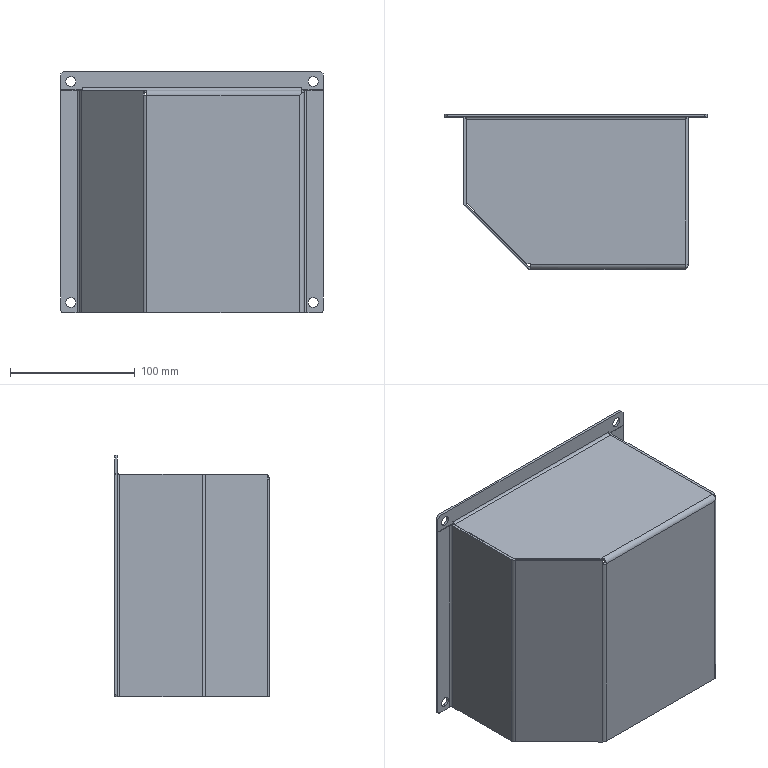Part | NX | features solid 2 | 1 solid | 68 faces | box 210 x 124 x 193 mm | volume 194772 mm3 | plane 43 | cylinder 25 | commonest cylinder face diameters 8 x15 4 x10